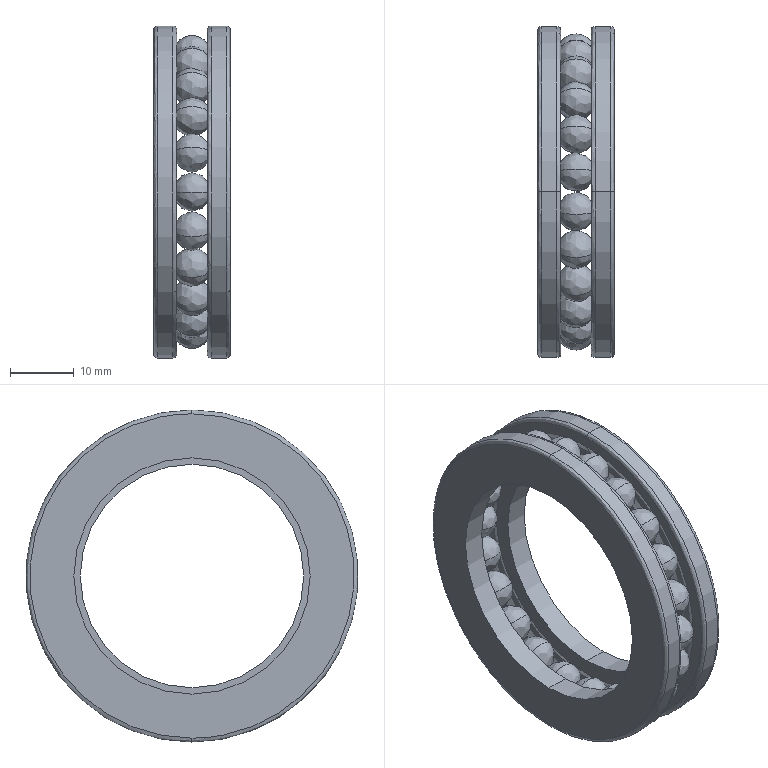Part | SolidWorks | features BaseBody 1 | 1 solid | 112 faces | box 12 x 52 x 52 mm | volume 10012 mm3 | spline 98 | cylinder 8 | plane 6 | commonest cylinder face diameters 52 x4 35 x2 37 x2